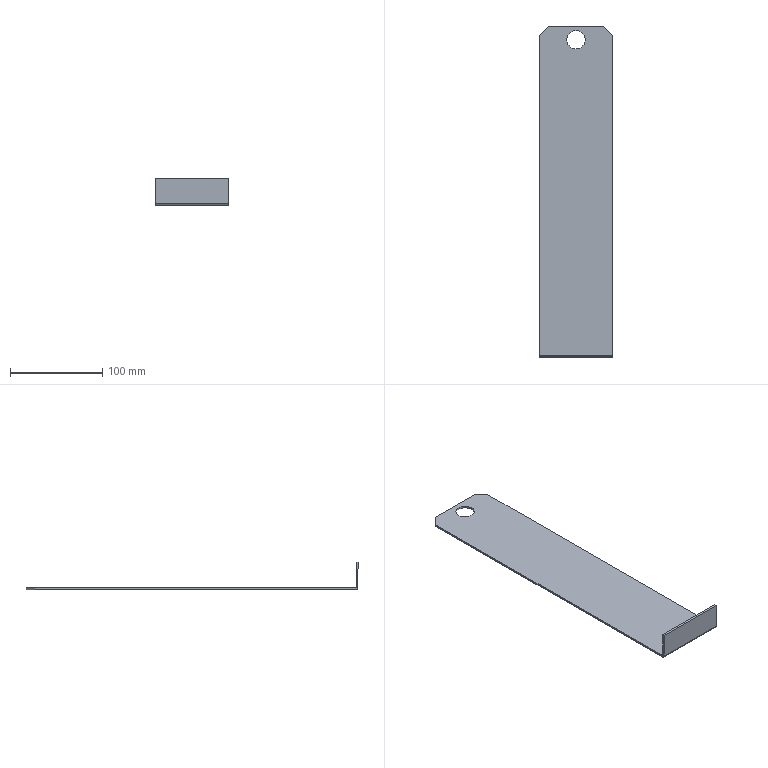Part | SolidWorks | features Chamfer 1, EdgeFlange 1, FlatPattern 1, ICE 1, SMBaseFlange 1, SheetMetal 1 | 1 solid | 18 faces | box 80 x 360 x 30 mm | volume 61132 mm3 | plane 14 | cylinder 4 | commonest cylinder face diameters 20 x2 1.473 x1 5.473 x1
STEP:
#1=CARTESIAN_POINT('',(-10.,165.,-2.));
#2=VERTEX_POINT('',#1);
#3=CARTESIAN_POINT('',(10.,165.,-2.));
#4=VERTEX_POINT('',#3);
#5=CARTESIAN_POINT('',(0.,165.,-2.));
#6=DIRECTION('',(0.,0.,1.));
#7=DIRECTION('',(1.,0.,0.));
#8=AXIS2_PLACEMENT_3D('',#5,#6,#7);
#9=CIRCLE('',#8,10.);
#10=EDGE_CURVE('',#2,#4,#9,.T.);
#11=ORIENTED_EDGE('',*,*,#10,.F.);
#12=CARTESIAN_POINT('',(-10.,165.,0.));
#13=VERTEX_POINT('',#12);
#14=CARTESIAN_POINT('',(-10.,165.,-2.));
#15=DIRECTION('',(0.,0.,1.));
#16=VECTOR('',#15,1000.);
#17=LINE('',#14,#16);
#18=EDGE_CURVE('',#2,#13,#17,.T.);
#19=ORIENTED_EDGE('',*,*,#18,.T.);
#20=CARTESIAN_POINT('',(10.,165.,0.));
#21=VERTEX_POINT('',#20);
#22=CARTESIAN_POINT('',(0.,165.,0.));
#23=DIRECTION('',(0.,0.,1.));
#24=DIRECTION('',(1.,0.,0.));
#25=AXIS2_PLACEMENT_3D('',#22,#23,#24);
#26=CIRCLE('',#25,10.);
#27=EDGE_CURVE('',#13,#21,#26,.T.);
#28=ORIENTED_EDGE('',*,*,#27,.T.);
#29=CARTESIAN_POINT('',(10.,165.,-2.));
#30=DIRECTION('',(0.,0.,1.));
#31=VECTOR('',#30,1000.);
#32=LINE('',#29,#31);
#33=EDGE_CURVE('',#4,#21,#32,.T.);
#34=ORIENTED_EDGE('',*,*,#33,.F.);
#35=EDGE_LOOP('',(#11,#19,#28,#34));
#36=FACE_OUTER_BOUND('',#35,.T.);
#37=CARTESIAN_POINT('',(0.,165.,-2.));
#38=DIRECTION('',(0.,0.,1.));
#39=DIRECTION('',(1.,0.,0.));
#40=AXIS2_PLACEMENT_3D('',#37,#38,#39);
#41=CYLINDRICAL_SURFACE('',#40,10.);
#42=ADVANCED_FACE('',(#36),#41,.F.);
#43=CARTESIAN_POINT('',(40.,-177.263,-2.));
#44=VERTEX_POINT('',#43);
#45=CARTESIAN_POINT('',(40.,170.,-2.));
#46=VERTEX_POINT('',#45);
#47=CARTESIAN_POINT('',(40.,-180.,-2.));
#48=DIRECTION('',(0.,1.,0.));
#49=VECTOR('',#48,1000.);
#50=LINE('',#47,#49);
#51=EDGE_CURVE('',#44,#46,#50,.T.);
#52=ORIENTED_EDGE('',*,*,#51,.T.);
#53=CARTESIAN_POINT('',(40.,170.,0.));
#54=VERTEX_POINT('',#53);
#55=CARTESIAN_POINT('',(40.,170.,-2.));
#56=DIRECTION('',(0.,0.,1.));
#57=VECTOR('',#56,1000.);
#58=LINE('',#55,#57);
#59=EDGE_CURVE('',#46,#54,#58,.T.);
#60=ORIENTED_EDGE('',*,*,#59,.T.);
#61=CARTESIAN_POINT('',(40.,-177.263,0.));
#62=VERTEX_POINT('',#61);
#63=CARTESIAN_POINT('',(40.,-180.,0.));
#64=DIRECTION('',(0.,1.,0.));
#65=VECTOR('',#64,1000.);
#66=LINE('',#63,#65);
#67=EDGE_CURVE('',#62,#54,#66,.T.);
#68=ORIENTED_EDGE('',*,*,#67,.F.);
#69=CARTESIAN_POINT('',(40.,-177.263,0.));
#70=DIRECTION('',(0.,0.,-1.));
#71=VECTOR('',#70,1000.);
#72=LINE('',#69,#71);
#73=EDGE_CURVE('',#62,#44,#72,.T.);
#74=ORIENTED_EDGE('',*,*,#73,.T.);
#75=EDGE_LOOP('',(#52,#60,#68,#74));
#76=FACE_OUTER_BOUND('',#75,.T.);
#77=CARTESIAN_POINT('',(40.,-180.,-2.));
#78=DIRECTION('',(1.,0.,0.));
#79=DIRECTION('',(0.,0.,-1.));
#80=AXIS2_PLACEMENT_3D('',#77,#78,#79);
#81=PLANE('',#80);
#82=ADVANCED_FACE('',(#76),#81,.T.);
#83=CARTESIAN_POINT('',(0.,165.,-2.));
#84=DIRECTION('',(0.,0.,1.));
#85=DIRECTION('',(1.,0.,0.));
#86=AXIS2_PLACEMENT_3D('',#83,#84,#85);
#87=CIRCLE('',#86,10.);
#88=EDGE_CURVE('',#4,#2,#87,.T.);
#89=ORIENTED_EDGE('',*,*,#88,.T.);
#90=ORIENTED_EDGE('',*,*,#10,.T.);
#91=EDGE_LOOP('',(#89,#90));
#92=FACE_BOUND('',#91,.T.);
#93=CARTESIAN_POINT('',(-40.,170.,-2.));
#94=VERTEX_POINT('',#93);
#95=CARTESIAN_POINT('',(-40.,-177.263,-2.));
#96=VERTEX_POINT('',#95);
#97=CARTESIAN_POINT('',(-40.,-180.,-2.));
#98=DIRECTION('',(0.,-1.,0.));
#99=VECTOR('',#98,1000.);
#100=LINE('',#97,#99);
#101=EDGE_CURVE('',#94,#96,#100,.T.);
#102=ORIENTED_EDGE('',*,*,#101,.F.);
#103=CARTESIAN_POINT('',(-30.,180.,-2.));
#104=VERTEX_POINT('',#103);
#105=CARTESIAN_POINT('',(-105.,105.,-2.));
#106=DIRECTION('',(0.7071,0.7071,0.));
#107=VECTOR('',#106,1000.);
#108=LINE('',#105,#107);
#109=EDGE_CURVE('',#94,#104,#108,.T.);
#110=ORIENTED_EDGE('',*,*,#109,.T.);
#111=CARTESIAN_POINT('',(30.,180.,-2.));
#112=VERTEX_POINT('',#111);
#113=CARTESIAN_POINT('',(-40.,180.,-2.));
#114=DIRECTION('',(-1.,0.,0.));
#115=VECTOR('',#114,1000.);
#116=LINE('',#113,#115);
#117=EDGE_CURVE('',#112,#104,#116,.T.);
#118=ORIENTED_EDGE('',*,*,#117,.F.);
#119=CARTESIAN_POINT('',(105.,105.,-2.));
#120=DIRECTION('',(0.7071,-0.7071,0.));
#121=VECTOR('',#120,1000.);
#122=LINE('',#119,#121);
#123=EDGE_CURVE('',#112,#46,#122,.T.);
#124=ORIENTED_EDGE('',*,*,#123,.T.);
#125=ORIENTED_EDGE('',*,*,#51,.F.);
#126=CARTESIAN_POINT('',(40.,-177.263,-2.));
#127=DIRECTION('',(-1.,0.,0.));
#128=VECTOR('',#127,1000.);
#129=LINE('',#126,#128);
#130=EDGE_CURVE('',#44,#96,#129,.T.);
#131=ORIENTED_EDGE('',*,*,#130,.T.);
#132=EDGE_LOOP('',(#102,#110,#118,#124,#125,#131));
#133=FACE_OUTER_BOUND('',#132,.T.);
#134=CARTESIAN_POINT('',(0.,0.,-2.));
#135=DIRECTION('',(0.,0.,-1.));
#136=DIRECTION('',(-1.,0.,0.));
#137=AXIS2_PLACEMENT_3D('',#134,#135,#136);
#138=PLANE('',#137);
#139=ADVANCED_FACE('',(#92,#133),#138,.T.);
#140=CARTESIAN_POINT('',(0.,165.,0.));
#141=DIRECTION('',(0.,0.,1.));
#142=DIRECTION('',(1.,0.,0.));
#143=AXIS2_PLACEMENT_3D('',#140,#141,#142);
#144=CIRCLE('',#143,10.);
#145=EDGE_CURVE('',#21,#13,#144,.T.);
#146=ORIENTED_EDGE('',*,*,#145,.F.);
#147=ORIENTED_EDGE('',*,*,#27,.F.);
#148=EDGE_LOOP('',(#146,#147));
#149=FACE_BOUND('',#148,.T.);
#150=CARTESIAN_POINT('',(30.,180.,0.));
#151=VERTEX_POINT('',#150);
#152=CARTESIAN_POINT('',(-30.,180.,0.));
#153=VERTEX_POINT('',#152);
#154=CARTESIAN_POINT('',(-40.,180.,0.));
#155=DIRECTION('',(-1.,0.,0.));
#156=VECTOR('',#155,1000.);
#157=LINE('',#154,#156);
#158=EDGE_CURVE('',#151,#153,#157,.T.);
#159=ORIENTED_EDGE('',*,*,#158,.T.);
#160=CARTESIAN_POINT('',(-40.,170.,0.));
#161=VERTEX_POINT('',#160);
#162=CARTESIAN_POINT('',(-30.,180.,0.));
#163=DIRECTION('',(-0.7071,-0.7071,0.));
#164=VECTOR('',#163,1000.);
#165=LINE('',#162,#164);
#166=EDGE_CURVE('',#153,#161,#165,.T.);
#167=ORIENTED_EDGE('',*,*,#166,.T.);
#168=CARTESIAN_POINT('',(-40.,-177.263,0.));
#169=VERTEX_POINT('',#168);
#170=CARTESIAN_POINT('',(-40.,-180.,0.));
#171=DIRECTION('',(0.,-1.,0.));
#172=VECTOR('',#171,1000.);
#173=LINE('',#170,#172);
#174=EDGE_CURVE('',#161,#169,#173,.T.);
#175=ORIENTED_EDGE('',*,*,#174,.T.);
#176=CARTESIAN_POINT('',(40.,-177.263,0.));
#177=DIRECTION('',(-1.,0.,0.));
#178=VECTOR('',#177,1000.);
#179=LINE('',#176,#178);
#180=EDGE_CURVE('',#62,#169,#179,.T.);
#181=ORIENTED_EDGE('',*,*,#180,.F.);
#182=ORIENTED_EDGE('',*,*,#67,.T.);
#183=CARTESIAN_POINT('',(40.,170.,0.));
#184=DIRECTION('',(-0.7071,0.7071,0.));
#185=VECTOR('',#184,1000.);
#186=LINE('',#183,#185);
#187=EDGE_CURVE('',#54,#151,#186,.T.);
#188=ORIENTED_EDGE('',*,*,#187,.T.);
#189=EDGE_LOOP('',(#159,#167,#175,#181,#182,#188));
#190=FACE_OUTER_BOUND('',#189,.T.);
#191=CARTESIAN_POINT('',(0.,0.,0.));
#192=DIRECTION('',(0.,0.,-1.));
#193=DIRECTION('',(-1.,0.,0.));
#194=AXIS2_PLACEMENT_3D('',#191,#192,#193);
#195=PLANE('',#194);
#196=ADVANCED_FACE('',(#149,#190),#195,.F.);
#197=ORIENTED_EDGE('',*,*,#174,.F.);
#198=CARTESIAN_POINT('',(-40.,170.,-2.));
#199=DIRECTION('',(0.,0.,-1.));
#200=VECTOR('',#199,1000.);
#201=LINE('',#198,#200);
#202=EDGE_CURVE('',#161,#94,#201,.T.);
#203=ORIENTED_EDGE('',*,*,#202,.T.);
#204=ORIENTED_EDGE('',*,*,#101,.T.);
#205=CARTESIAN_POINT('',(-40.,-177.263,0.));
#206=DIRECTION('',(0.,0.,-1.));
#207=VECTOR('',#206,1000.);
#208=LINE('',#205,#207);
#209=EDGE_CURVE('',#169,#96,#208,.T.);
#210=ORIENTED_EDGE('',*,*,#209,.F.);
#211=EDGE_LOOP('',(#197,#203,#204,#210));
#212=FACE_OUTER_BOUND('',#211,.T.);
#213=CARTESIAN_POINT('',(-40.,-180.,-2.));
#214=DIRECTION('',(-1.,0.,0.));
#215=DIRECTION('',(0.,0.,1.));
#216=AXIS2_PLACEMENT_3D('',#213,#214,#215);
#217=PLANE('',#216);
#218=ADVANCED_FACE('',(#212),#217,.T.);
#219=ORIENTED_EDGE('',*,*,#117,.T.);
#220=CARTESIAN_POINT('',(-30.,180.,-2.));
#221=DIRECTION('',(0.,0.,1.));
#222=VECTOR('',#221,1000.);
#223=LINE('',#220,#222);
#224=EDGE_CURVE('',#104,#153,#223,.T.);
#225=ORIENTED_EDGE('',*,*,#224,.T.);
#226=ORIENTED_EDGE('',*,*,#158,.F.);
#227=CARTESIAN_POINT('',(30.,180.,-2.));
#228=DIRECTION('',(0.,0.,-1.));
#229=VECTOR('',#228,1000.);
#230=LINE('',#227,#229);
#231=EDGE_CURVE('',#151,#112,#230,.T.);
#232=ORIENTED_EDGE('',*,*,#231,.T.);
#233=EDGE_LOOP('',(#219,#225,#226,#232));
#234=FACE_OUTER_BOUND('',#233,.T.);
#235=CARTESIAN_POINT('',(-40.,180.,-2.));
#236=DIRECTION('',(0.,1.,0.));
#237=DIRECTION('',(0.,0.,1.));
#238=AXIS2_PLACEMENT_3D('',#235,#236,#237);
#239=PLANE('',#238);
#240=ADVANCED_FACE('',(#234),#239,.T.);
#241=CARTESIAN_POINT('',(-40.,-178.,0.7366));
#242=VERTEX_POINT('',#241);
#243=CARTESIAN_POINT('',(-40.,-180.,0.7366));
#244=VERTEX_POINT('',#243);
#245=CARTESIAN_POINT('',(-40.,-180.,0.7366));
#246=DIRECTION('',(0.,-1.,0.));
#247=VECTOR('',#246,1000.);
#248=LINE('',#245,#247);
#249=EDGE_CURVE('',#242,#244,#248,.T.);
#250=ORIENTED_EDGE('',*,*,#249,.F.);
#251=CARTESIAN_POINT('',(-40.,-177.263,0.7366));
#252=DIRECTION('',(-1.,0.,0.));
#253=DIRECTION('',(0.,0.,-1.));
#254=AXIS2_PLACEMENT_3D('',#251,#252,#253);
#255=CIRCLE('',#254,0.7366);
#256=EDGE_CURVE('',#169,#242,#255,.T.);
#257=ORIENTED_EDGE('',*,*,#256,.F.);
#258=ORIENTED_EDGE('',*,*,#209,.T.);
#259=CARTESIAN_POINT('',(-40.,-177.263,0.7366));
#260=DIRECTION('',(-1.,0.,0.));
#261=DIRECTION('',(0.,0.,-1.));
#262=AXIS2_PLACEMENT_3D('',#259,#260,#261);
#263=CIRCLE('',#262,2.737);
#264=EDGE_CURVE('',#96,#244,#263,.T.);
#265=ORIENTED_EDGE('',*,*,#264,.T.);
#266=EDGE_LOOP('',(#250,#257,#258,#265));
#267=FACE_OUTER_BOUND('',#266,.T.);
#268=CARTESIAN_POINT('',(-40.,-177.263,0.7366));
#269=DIRECTION('',(-1.,0.,0.));
#270=DIRECTION('',(0.,0.,1.));
#271=AXIS2_PLACEMENT_3D('',#268,#269,#270);
#272=PLANE('',#271);
#273=ADVANCED_FACE('',(#267),#272,.T.);
#274=CARTESIAN_POINT('',(40.,-178.,0.7366));
#275=VERTEX_POINT('',#274);
#276=CARTESIAN_POINT('',(40.,-177.263,0.7366));
#277=DIRECTION('',(1.,0.,0.));
#278=DIRECTION('',(0.,0.,-1.));
#279=AXIS2_PLACEMENT_3D('',#276,#277,#278);
#280=CIRCLE('',#279,0.7366);
#281=EDGE_CURVE('',#275,#62,#280,.T.);
#282=ORIENTED_EDGE('',*,*,#281,.F.);
#283=CARTESIAN_POINT('',(40.,-180.,0.7366));
#284=VERTEX_POINT('',#283);
#285=CARTESIAN_POINT('',(40.,-178.,0.7366));
#286=DIRECTION('',(0.,-1.,0.));
#287=VECTOR('',#286,1000.);
#288=LINE('',#285,#287);
#289=EDGE_CURVE('',#275,#284,#288,.T.);
#290=ORIENTED_EDGE('',*,*,#289,.T.);
#291=CARTESIAN_POINT('',(40.,-177.263,0.7366));
#292=DIRECTION('',(1.,0.,0.));
#293=DIRECTION('',(0.,0.,-1.));
#294=AXIS2_PLACEMENT_3D('',#291,#292,#293);
#295=CIRCLE('',#294,2.737);
#296=EDGE_CURVE('',#284,#44,#295,.T.);
#297=ORIENTED_EDGE('',*,*,#296,.T.);
#298=ORIENTED_EDGE('',*,*,#73,.F.);
#299=EDGE_LOOP('',(#282,#290,#297,#298));
#300=FACE_OUTER_BOUND('',#299,.T.);
#301=CARTESIAN_POINT('',(40.,-177.263,0.7366));
#302=DIRECTION('',(-1.,0.,0.));
#303=DIRECTION('',(0.,0.,1.));
#304=AXIS2_PLACEMENT_3D('',#301,#302,#303);
#305=PLANE('',#304);
#306=ADVANCED_FACE('',(#300),#305,.F.);
#307=ORIENTED_EDGE('',*,*,#130,.F.);
#308=ORIENTED_EDGE('',*,*,#296,.F.);
#309=CARTESIAN_POINT('',(-40.,-180.,0.7366));
#310=DIRECTION('',(-1.,0.,0.));
#311=VECTOR('',#310,1000.);
#312=LINE('',#309,#311);
#313=EDGE_CURVE('',#284,#244,#312,.T.);
#314=ORIENTED_EDGE('',*,*,#313,.T.);
#315=ORIENTED_EDGE('',*,*,#264,.F.);
#316=EDGE_LOOP('',(#307,#308,#314,#315));
#317=FACE_OUTER_BOUND('',#316,.T.);
#318=CARTESIAN_POINT('',(40.,-177.263,0.7366));
#319=DIRECTION('',(1.,0.,0.));
#320=DIRECTION('',(0.,-1.,0.));
#321=AXIS2_PLACEMENT_3D('',#318,#319,#320);
#322=CYLINDRICAL_SURFACE('',#321,2.737);
#323=ADVANCED_FACE('',(#317),#322,.T.);
#324=ORIENTED_EDGE('',*,*,#180,.T.);
#325=ORIENTED_EDGE('',*,*,#256,.T.);
#326=CARTESIAN_POINT('',(-40.,-178.,0.7366));
#327=DIRECTION('',(1.,0.,0.));
#328=VECTOR('',#327,1000.);
#329=LINE('',#326,#328);
#330=EDGE_CURVE('',#242,#275,#329,.T.);
#331=ORIENTED_EDGE('',*,*,#330,.T.);
#332=ORIENTED_EDGE('',*,*,#281,.T.);
#333=EDGE_LOOP('',(#324,#325,#331,#332));
#334=FACE_OUTER_BOUND('',#333,.T.);
#335=CARTESIAN_POINT('',(40.,-177.263,0.7366));
#336=DIRECTION('',(1.,0.,0.));
#337=DIRECTION('',(0.,-1.,0.));
#338=AXIS2_PLACEMENT_3D('',#335,#336,#337);
#339=CYLINDRICAL_SURFACE('',#338,0.7366);
#340=ADVANCED_FACE('',(#334),#339,.F.);
#341=ORIENTED_EDGE('',*,*,#249,.T.);
#342=CARTESIAN_POINT('',(-40.,-180.,28.));
#343=VERTEX_POINT('',#342);
#344=CARTESIAN_POINT('',(-40.,-180.,0.));
#345=DIRECTION('',(0.,0.,-1.));
#346=VECTOR('',#345,1000.);
#347=LINE('',#344,#346);
#348=EDGE_CURVE('',#343,#244,#347,.T.);
#349=ORIENTED_EDGE('',*,*,#348,.F.);
#350=CARTESIAN_POINT('',(-40.,-178.,28.));
#351=VERTEX_POINT('',#350);
#352=CARTESIAN_POINT('',(-40.,-180.,28.));
#353=DIRECTION('',(0.,1.,0.));
#354=VECTOR('',#353,1000.);
#355=LINE('',#352,#354);
#356=EDGE_CURVE('',#343,#351,#355,.T.);
#357=ORIENTED_EDGE('',*,*,#356,.T.);
#358=CARTESIAN_POINT('',(-40.,-178.,0.));
#359=DIRECTION('',(0.,0.,-1.));
#360=VECTOR('',#359,1000.);
#361=LINE('',#358,#360);
#362=EDGE_CURVE('',#351,#242,#361,.T.);
#363=ORIENTED_EDGE('',*,*,#362,.T.);
#364=EDGE_LOOP('',(#341,#349,#357,#363));
#365=FACE_OUTER_BOUND('',#364,.T.);
#366=CARTESIAN_POINT('',(-40.,-180.,0.));
#367=DIRECTION('',(1.,0.,0.));
#368=DIRECTION('',(0.,0.,-1.));
#369=AXIS2_PLACEMENT_3D('',#366,#367,#368);
#370=PLANE('',#369);
#371=ADVANCED_FACE('',(#365),#370,.F.);
#372=ORIENTED_EDGE('',*,*,#289,.F.);
#373=CARTESIAN_POINT('',(40.,-178.,28.));
#374=VERTEX_POINT('',#373);
#375=CARTESIAN_POINT('',(40.,-178.,28.));
#376=DIRECTION('',(0.,0.,1.));
#377=VECTOR('',#376,1000.);
#378=LINE('',#375,#377);
#379=EDGE_CURVE('',#275,#374,#378,.T.);
#380=ORIENTED_EDGE('',*,*,#379,.T.);
#381=CARTESIAN_POINT('',(40.,-180.,28.));
#382=VERTEX_POINT('',#381);
#383=CARTESIAN_POINT('',(40.,-180.,28.));
#384=DIRECTION('',(0.,1.,0.));
#385=VECTOR('',#384,1000.);
#386=LINE('',#383,#385);
#387=EDGE_CURVE('',#382,#374,#386,.T.);
#388=ORIENTED_EDGE('',*,*,#387,.F.);
#389=CARTESIAN_POINT('',(40.,-180.,0.));
#390=DIRECTION('',(0.,0.,1.));
#391=VECTOR('',#390,1000.);
#392=LINE('',#389,#391);
#393=EDGE_CURVE('',#284,#382,#392,.T.);
#394=ORIENTED_EDGE('',*,*,#393,.F.);
#395=EDGE_LOOP('',(#372,#380,#388,#394));
#396=FACE_OUTER_BOUND('',#395,.T.);
#397=CARTESIAN_POINT('',(40.,-180.,28.));
#398=DIRECTION('',(-1.,0.,0.));
#399=DIRECTION('',(0.,0.,1.));
#400=AXIS2_PLACEMENT_3D('',#397,#398,#399);
#401=PLANE('',#400);
#402=ADVANCED_FACE('',(#396),#401,.F.);
#403=ORIENTED_EDGE('',*,*,#313,.F.);
#404=ORIENTED_EDGE('',*,*,#393,.T.);
#405=CARTESIAN_POINT('',(0.,-180.,28.));
#406=DIRECTION('',(-1.,0.,0.));
#407=VECTOR('',#406,1000.);
#408=LINE('',#405,#407);
#409=EDGE_CURVE('',#382,#343,#408,.T.);
#410=ORIENTED_EDGE('',*,*,#409,.T.);
#411=ORIENTED_EDGE('',*,*,#348,.T.);
#412=EDGE_LOOP('',(#403,#404,#410,#411));
#413=FACE_OUTER_BOUND('',#412,.T.);
#414=CARTESIAN_POINT('',(0.,-180.,0.));
#415=DIRECTION('',(0.,1.,0.));
#416=DIRECTION('',(0.,0.,1.));
#417=AXIS2_PLACEMENT_3D('',#414,#415,#416);
#418=PLANE('',#417);
#419=ADVANCED_FACE('',(#413),#418,.F.);
#420=ORIENTED_EDGE('',*,*,#379,.F.);
#421=ORIENTED_EDGE('',*,*,#330,.F.);
#422=ORIENTED_EDGE('',*,*,#362,.F.);
#423=CARTESIAN_POINT('',(-40.,-178.,28.));
#424=DIRECTION('',(-1.,0.,0.));
#425=VECTOR('',#424,1000.);
#426=LINE('',#423,#425);
#427=EDGE_CURVE('',#374,#351,#426,.T.);
#428=ORIENTED_EDGE('',*,*,#427,.F.);
#429=EDGE_LOOP('',(#420,#421,#422,#428));
#430=FACE_OUTER_BOUND('',#429,.T.);
#431=CARTESIAN_POINT('',(0.,-178.,0.));
#432=DIRECTION('',(0.,1.,0.));
#433=DIRECTION('',(0.,0.,1.));
#434=AXIS2_PLACEMENT_3D('',#431,#432,#433);
#435=PLANE('',#434);
#436=ADVANCED_FACE('',(#430),#435,.T.);
#437=ORIENTED_EDGE('',*,*,#427,.T.);
#438=ORIENTED_EDGE('',*,*,#356,.F.);
#439=ORIENTED_EDGE('',*,*,#409,.F.);
#440=ORIENTED_EDGE('',*,*,#387,.T.);
#441=EDGE_LOOP('',(#437,#438,#439,#440));
#442=FACE_OUTER_BOUND('',#441,.T.);
#443=CARTESIAN_POINT('',(-40.,-180.,28.));
#444=DIRECTION('',(0.,0.,-1.));
#445=DIRECTION('',(0.,1.,0.));
#446=AXIS2_PLACEMENT_3D('',#443,#444,#445);
#447=PLANE('',#446);
#448=ADVANCED_FACE('',(#442),#447,.F.);
#449=ORIENTED_EDGE('',*,*,#18,.F.);
#450=ORIENTED_EDGE('',*,*,#88,.F.);
#451=ORIENTED_EDGE('',*,*,#33,.T.);
#452=ORIENTED_EDGE('',*,*,#145,.T.);
#453=EDGE_LOOP('',(#449,#450,#451,#452));
#454=FACE_OUTER_BOUND('',#453,.T.);
#455=CARTESIAN_POINT('',(0.,165.,-2.));
#456=DIRECTION('',(0.,0.,1.));
#457=DIRECTION('',(1.,0.,0.));
#458=AXIS2_PLACEMENT_3D('',#455,#456,#457);
#459=CYLINDRICAL_SURFACE('',#458,10.);
#460=ADVANCED_FACE('',(#454),#459,.F.);
#461=ORIENTED_EDGE('',*,*,#109,.F.);
#462=ORIENTED_EDGE('',*,*,#202,.F.);
#463=ORIENTED_EDGE('',*,*,#166,.F.);
#464=ORIENTED_EDGE('',*,*,#224,.F.);
#465=EDGE_LOOP('',(#461,#462,#463,#464));
#466=FACE_OUTER_BOUND('',#465,.T.);
#467=CARTESIAN_POINT('',(-30.,180.,-2.));
#468=DIRECTION('',(0.7071,-0.7071,0.));
#469=DIRECTION('',(0.,0.,1.));
#470=AXIS2_PLACEMENT_3D('',#467,#468,#469);
#471=PLANE('',#470);
#472=ADVANCED_FACE('',(#466),#471,.F.);
#473=ORIENTED_EDGE('',*,*,#123,.F.);
#474=ORIENTED_EDGE('',*,*,#231,.F.);
#475=ORIENTED_EDGE('',*,*,#187,.F.);
#476=ORIENTED_EDGE('',*,*,#59,.F.);
#477=EDGE_LOOP('',(#473,#474,#475,#476));
#478=FACE_OUTER_BOUND('',#477,.T.);
#479=CARTESIAN_POINT('',(40.,170.,-2.));
#480=DIRECTION('',(-0.7071,-0.7071,0.));
#481=DIRECTION('',(0.,0.,1.));
#482=AXIS2_PLACEMENT_3D('',#479,#480,#481);
#483=PLANE('',#482);
#484=ADVANCED_FACE('',(#478),#483,.F.);
#485=CLOSED_SHELL('',(#42,#82,#139,#196,#218,#240,#273,#306,#323,#340,#371,#402,#419,#436,#448,#460,#472,#484));
#486=MANIFOLD_SOLID_BREP('',#485);
#487=CARTESIAN_POINT('',(0.,0.,0.));
#488=DIRECTION('',(0.,0.,1.));
#489=DIRECTION('',(1.,0.,0.));
#490=AXIS2_PLACEMENT_3D('',#487,#488,#489);
#491=(LENGTH_UNIT()NAMED_UNIT(*)SI_UNIT(.MILLI.,.METRE.));
#492=UNCERTAINTY_MEASURE_WITH_UNIT(LENGTH_MEASURE(0.00001),#491,'','');
#493=(NAMED_UNIT(*)PLANE_ANGLE_UNIT()SI_UNIT($,.RADIAN.));
#494=(NAMED_UNIT(*)SI_UNIT($,.STERADIAN.)SOLID_ANGLE_UNIT());
#495=(GEOMETRIC_REPRESENTATION_CONTEXT(3)GLOBAL_UNCERTAINTY_ASSIGNED_CONTEXT((#492))GLOBAL_UNIT_ASSIGNED_CONTEXT((#491,#493,#494))REPRESENTATION_CONTEXT('',''));
#496=ADVANCED_BREP_SHAPE_REPRESENTATION('',(#486,#490),#495);